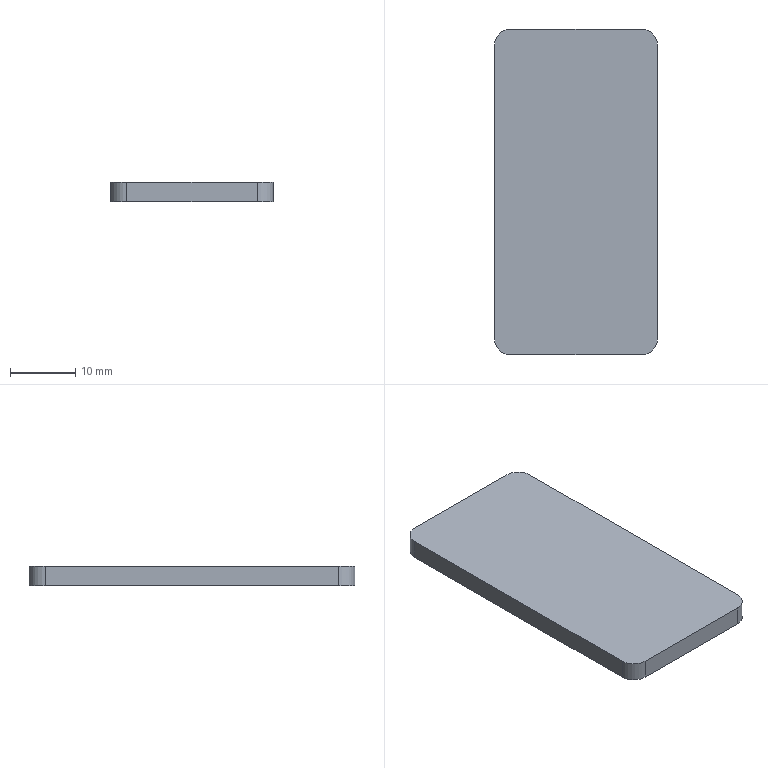Part | STEP file | 7100518 | 1 solid | 10 faces | box 25 x 50 x 3 mm | volume 3734 mm3 | plane 6 | cylinder 4 | commonest cylinder face diameters 5 x4
STEP:
#1=CARTESIAN_POINT('',(0.,0.,0.));
#2=DIRECTION('',(0.,0.,1.));
#3=DIRECTION('',(1.,0.,0.));
#4=AXIS2_PLACEMENT_3D('',#1,#2,#3);
#5=CARTESIAN_POINT('',(10.,-25.,0.));
#6=VERTEX_POINT('',#5);
#7=CARTESIAN_POINT('',(12.5,-22.5,0.));
#8=VERTEX_POINT('',#7);
#9=CARTESIAN_POINT('',(10.,-22.5,0.));
#10=DIRECTION('',(0.,0.,1.));
#11=DIRECTION('',(1.,0.,0.));
#12=AXIS2_PLACEMENT_3D('',#9,#10,#11);
#13=CIRCLE('',#12,2.5);
#14=CARTESIAN_POINT('',(10.,-22.5,3.));
#15=DIRECTION('',(0.,0.,-1.));
#16=DIRECTION('',(-1.,0.,0.));
#17=AXIS2_PLACEMENT_3D('',#14,#15,#16);
#18=CYLINDRICAL_SURFACE('',#17,2.5);
#19=CARTESIAN_POINT('',(9.425,3.));
#20=DIRECTION('',(-1.,0.));
#21=VECTOR('',#20,1.);
#22=LINE('',#19,#21);
#23=(GEOMETRIC_REPRESENTATION_CONTEXT(2)PARAMETRIC_REPRESENTATION_CONTEXT()REPRESENTATION_CONTEXT('',''));
#24=DEFINITIONAL_REPRESENTATION('',(#22),#23);
#25=PCURVE('',#18,#24);
#26=CARTESIAN_POINT('',(10.,-22.5,0.));
#27=DIRECTION('',(0.,0.,1.));
#28=DIRECTION('',(1.,0.,0.));
#29=AXIS2_PLACEMENT_3D('',#26,#27,#28);
#30=PLANE('',#29);
#31=CARTESIAN_POINT('',(0.,0.));
#32=DIRECTION('',(1.,0.));
#33=AXIS2_PLACEMENT_2D('',#31,#32);
#34=CIRCLE('',#33,2.5);
#35=(GEOMETRIC_REPRESENTATION_CONTEXT(2)PARAMETRIC_REPRESENTATION_CONTEXT()REPRESENTATION_CONTEXT('',''));
#36=DEFINITIONAL_REPRESENTATION('',(#34),#35);
#37=PCURVE('',#30,#36);
#38=SURFACE_CURVE('',#13,(#25,#37),.PCURVE_S1.);
#39=EDGE_CURVE('',#6,#8,#38,.T.);
#40=ORIENTED_EDGE('',*,*,#39,.T.);
#41=CARTESIAN_POINT('',(12.5,-22.5,3.));
#42=VERTEX_POINT('',#41);
#43=CARTESIAN_POINT('',(12.5,-22.5,3.));
#44=DIRECTION('',(0.,0.,-1.));
#45=VECTOR('',#44,1.);
#46=LINE('',#43,#45);
#47=CARTESIAN_POINT('',(3.142,0.));
#48=DIRECTION('',(0.,1.));
#49=VECTOR('',#48,1.);
#50=LINE('',#47,#49);
#51=(GEOMETRIC_REPRESENTATION_CONTEXT(2)PARAMETRIC_REPRESENTATION_CONTEXT()REPRESENTATION_CONTEXT('',''));
#52=DEFINITIONAL_REPRESENTATION('',(#50),#51);
#53=PCURVE('',#18,#52);
#54=CARTESIAN_POINT('',(12.5,22.5,3.));
#55=DIRECTION('',(-1.,0.,0.));
#56=DIRECTION('',(0.,-1.,0.));
#57=AXIS2_PLACEMENT_3D('',#54,#55,#56);
#58=PLANE('',#57);
#59=CARTESIAN_POINT('',(45.,0.));
#60=DIRECTION('',(0.,-1.));
#61=VECTOR('',#60,1.);
#62=LINE('',#59,#61);
#63=(GEOMETRIC_REPRESENTATION_CONTEXT(2)PARAMETRIC_REPRESENTATION_CONTEXT()REPRESENTATION_CONTEXT('',''));
#64=DEFINITIONAL_REPRESENTATION('',(#62),#63);
#65=PCURVE('',#58,#64);
#66=SURFACE_CURVE('',#46,(#53,#65),.PCURVE_S1.);
#67=EDGE_CURVE('',#42,#8,#66,.T.);
#68=ORIENTED_EDGE('',*,*,#67,.F.);
#69=CARTESIAN_POINT('',(10.,-25.,3.));
#70=VERTEX_POINT('',#69);
#71=CARTESIAN_POINT('',(10.,-22.5,3.));
#72=DIRECTION('',(0.,0.,1.));
#73=DIRECTION('',(1.,0.,0.));
#74=AXIS2_PLACEMENT_3D('',#71,#72,#73);
#75=CIRCLE('',#74,2.5);
#76=CARTESIAN_POINT('',(9.425,0.));
#77=DIRECTION('',(-1.,0.));
#78=VECTOR('',#77,1.);
#79=LINE('',#76,#78);
#80=(GEOMETRIC_REPRESENTATION_CONTEXT(2)PARAMETRIC_REPRESENTATION_CONTEXT()REPRESENTATION_CONTEXT('',''));
#81=DEFINITIONAL_REPRESENTATION('',(#79),#80);
#82=PCURVE('',#18,#81);
#83=CARTESIAN_POINT('',(10.,-22.5,3.));
#84=DIRECTION('',(0.,0.,1.));
#85=DIRECTION('',(1.,0.,0.));
#86=AXIS2_PLACEMENT_3D('',#83,#84,#85);
#87=PLANE('',#86);
#88=CARTESIAN_POINT('',(0.,0.));
#89=DIRECTION('',(1.,0.));
#90=AXIS2_PLACEMENT_2D('',#88,#89);
#91=CIRCLE('',#90,2.5);
#92=(GEOMETRIC_REPRESENTATION_CONTEXT(2)PARAMETRIC_REPRESENTATION_CONTEXT()REPRESENTATION_CONTEXT('',''));
#93=DEFINITIONAL_REPRESENTATION('',(#91),#92);
#94=PCURVE('',#87,#93);
#95=SURFACE_CURVE('',#75,(#82,#94),.PCURVE_S1.);
#96=EDGE_CURVE('',#70,#42,#95,.T.);
#97=ORIENTED_EDGE('',*,*,#96,.F.);
#98=CARTESIAN_POINT('',(10.,-25.,3.));
#99=DIRECTION('',(0.,0.,-1.));
#100=VECTOR('',#99,1.);
#101=LINE('',#98,#100);
#102=CARTESIAN_POINT('',(4.712,0.));
#103=DIRECTION('',(0.,1.));
#104=VECTOR('',#103,1.);
#105=LINE('',#102,#104);
#106=(GEOMETRIC_REPRESENTATION_CONTEXT(2)PARAMETRIC_REPRESENTATION_CONTEXT()REPRESENTATION_CONTEXT('',''));
#107=DEFINITIONAL_REPRESENTATION('',(#105),#106);
#108=PCURVE('',#18,#107);
#109=CARTESIAN_POINT('',(-10.,-25.,3.));
#110=DIRECTION('',(0.,1.,0.));
#111=DIRECTION('',(-1.,0.,0.));
#112=AXIS2_PLACEMENT_3D('',#109,#110,#111);
#113=PLANE('',#112);
#114=CARTESIAN_POINT('',(-20.,0.));
#115=DIRECTION('',(0.,-1.));
#116=VECTOR('',#115,1.);
#117=LINE('',#114,#116);
#118=(GEOMETRIC_REPRESENTATION_CONTEXT(2)PARAMETRIC_REPRESENTATION_CONTEXT()REPRESENTATION_CONTEXT('',''));
#119=DEFINITIONAL_REPRESENTATION('',(#117),#118);
#120=PCURVE('',#113,#119);
#121=SURFACE_CURVE('',#101,(#108,#120),.PCURVE_S1.);
#122=EDGE_CURVE('',#70,#6,#121,.T.);
#123=ORIENTED_EDGE('',*,*,#122,.T.);
#124=EDGE_LOOP('',(#40,#68,#97,#123));
#125=FACE_BOUND('',#124,.T.);
#126=ADVANCED_FACE('',(#125),#18,.T.);
#127=CARTESIAN_POINT('',(12.5,22.5,0.));
#128=VERTEX_POINT('',#127);
#129=CARTESIAN_POINT('',(12.5,22.5,0.));
#130=DIRECTION('',(0.,1.,0.));
#131=VECTOR('',#130,1.);
#132=LINE('',#129,#131);
#133=CARTESIAN_POINT('',(0.,-3.));
#134=DIRECTION('',(-1.,0.));
#135=VECTOR('',#134,1.);
#136=LINE('',#133,#135);
#137=(GEOMETRIC_REPRESENTATION_CONTEXT(2)PARAMETRIC_REPRESENTATION_CONTEXT()REPRESENTATION_CONTEXT('',''));
#138=DEFINITIONAL_REPRESENTATION('',(#136),#137);
#139=PCURVE('',#58,#138);
#140=CARTESIAN_POINT('',(2.5,45.));
#141=DIRECTION('',(0.,1.));
#142=VECTOR('',#141,1.);
#143=LINE('',#140,#142);
#144=(GEOMETRIC_REPRESENTATION_CONTEXT(2)PARAMETRIC_REPRESENTATION_CONTEXT()REPRESENTATION_CONTEXT('',''));
#145=DEFINITIONAL_REPRESENTATION('',(#143),#144);
#146=PCURVE('',#30,#145);
#147=SURFACE_CURVE('',#132,(#139,#146),.PCURVE_S1.);
#148=EDGE_CURVE('',#8,#128,#147,.T.);
#149=ORIENTED_EDGE('',*,*,#148,.T.);
#150=CARTESIAN_POINT('',(12.5,22.5,3.));
#151=VERTEX_POINT('',#150);
#152=CARTESIAN_POINT('',(12.5,22.5,3.));
#153=DIRECTION('',(0.,0.,-1.));
#154=VECTOR('',#153,1.);
#155=LINE('',#152,#154);
#156=CARTESIAN_POINT('',(0.,0.));
#157=DIRECTION('',(0.,-1.));
#158=VECTOR('',#157,1.);
#159=LINE('',#156,#158);
#160=(GEOMETRIC_REPRESENTATION_CONTEXT(2)PARAMETRIC_REPRESENTATION_CONTEXT()REPRESENTATION_CONTEXT('',''));
#161=DEFINITIONAL_REPRESENTATION('',(#159),#160);
#162=PCURVE('',#58,#161);
#163=CARTESIAN_POINT('',(10.,22.5,3.));
#164=DIRECTION('',(0.,0.,-1.));
#165=DIRECTION('',(-1.,0.,0.));
#166=AXIS2_PLACEMENT_3D('',#163,#164,#165);
#167=CYLINDRICAL_SURFACE('',#166,2.5);
#168=CARTESIAN_POINT('',(3.142,0.));
#169=DIRECTION('',(0.,1.));
#170=VECTOR('',#169,1.);
#171=LINE('',#168,#170);
#172=(GEOMETRIC_REPRESENTATION_CONTEXT(2)PARAMETRIC_REPRESENTATION_CONTEXT()REPRESENTATION_CONTEXT('',''));
#173=DEFINITIONAL_REPRESENTATION('',(#171),#172);
#174=PCURVE('',#167,#173);
#175=SURFACE_CURVE('',#155,(#162,#174),.PCURVE_S1.);
#176=EDGE_CURVE('',#151,#128,#175,.T.);
#177=ORIENTED_EDGE('',*,*,#176,.F.);
#178=CARTESIAN_POINT('',(12.5,22.5,3.));
#179=DIRECTION('',(0.,1.,0.));
#180=VECTOR('',#179,1.);
#181=LINE('',#178,#180);
#182=CARTESIAN_POINT('',(0.,0.));
#183=DIRECTION('',(-1.,0.));
#184=VECTOR('',#183,1.);
#185=LINE('',#182,#184);
#186=(GEOMETRIC_REPRESENTATION_CONTEXT(2)PARAMETRIC_REPRESENTATION_CONTEXT()REPRESENTATION_CONTEXT('',''));
#187=DEFINITIONAL_REPRESENTATION('',(#185),#186);
#188=PCURVE('',#58,#187);
#189=CARTESIAN_POINT('',(2.5,45.));
#190=DIRECTION('',(0.,1.));
#191=VECTOR('',#190,1.);
#192=LINE('',#189,#191);
#193=(GEOMETRIC_REPRESENTATION_CONTEXT(2)PARAMETRIC_REPRESENTATION_CONTEXT()REPRESENTATION_CONTEXT('',''));
#194=DEFINITIONAL_REPRESENTATION('',(#192),#193);
#195=PCURVE('',#87,#194);
#196=SURFACE_CURVE('',#181,(#188,#195),.PCURVE_S1.);
#197=EDGE_CURVE('',#42,#151,#196,.T.);
#198=ORIENTED_EDGE('',*,*,#197,.F.);
#199=ORIENTED_EDGE('',*,*,#67,.T.);
#200=EDGE_LOOP('',(#149,#177,#198,#199));
#201=FACE_BOUND('',#200,.T.);
#202=ADVANCED_FACE('',(#201),#58,.F.);
#203=CARTESIAN_POINT('',(10.,25.,0.));
#204=VERTEX_POINT('',#203);
#205=CARTESIAN_POINT('',(10.,22.5,0.));
#206=DIRECTION('',(0.,0.,1.));
#207=DIRECTION('',(-1.,0.,0.));
#208=AXIS2_PLACEMENT_3D('',#205,#206,#207);
#209=CIRCLE('',#208,2.5);
#210=CARTESIAN_POINT('',(6.283,3.));
#211=DIRECTION('',(-1.,0.));
#212=VECTOR('',#211,1.);
#213=LINE('',#210,#212);
#214=(GEOMETRIC_REPRESENTATION_CONTEXT(2)PARAMETRIC_REPRESENTATION_CONTEXT()REPRESENTATION_CONTEXT('',''));
#215=DEFINITIONAL_REPRESENTATION('',(#213),#214);
#216=PCURVE('',#167,#215);
#217=CARTESIAN_POINT('',(0.,45.));
#218=DIRECTION('',(-1.,0.));
#219=AXIS2_PLACEMENT_2D('',#217,#218);
#220=CIRCLE('',#219,2.5);
#221=(GEOMETRIC_REPRESENTATION_CONTEXT(2)PARAMETRIC_REPRESENTATION_CONTEXT()REPRESENTATION_CONTEXT('',''));
#222=DEFINITIONAL_REPRESENTATION('',(#220),#221);
#223=PCURVE('',#30,#222);
#224=SURFACE_CURVE('',#209,(#216,#223),.PCURVE_S1.);
#225=EDGE_CURVE('',#128,#204,#224,.T.);
#226=ORIENTED_EDGE('',*,*,#225,.T.);
#227=CARTESIAN_POINT('',(10.,25.,3.));
#228=VERTEX_POINT('',#227);
#229=CARTESIAN_POINT('',(10.,25.,3.));
#230=DIRECTION('',(0.,0.,-1.));
#231=VECTOR('',#230,1.);
#232=LINE('',#229,#231);
#233=CARTESIAN_POINT('',(1.571,0.));
#234=DIRECTION('',(0.,1.));
#235=VECTOR('',#234,1.);
#236=LINE('',#233,#235);
#237=(GEOMETRIC_REPRESENTATION_CONTEXT(2)PARAMETRIC_REPRESENTATION_CONTEXT()REPRESENTATION_CONTEXT('',''));
#238=DEFINITIONAL_REPRESENTATION('',(#236),#237);
#239=PCURVE('',#167,#238);
#240=CARTESIAN_POINT('',(-10.,25.,3.));
#241=DIRECTION('',(0.,-1.,0.));
#242=DIRECTION('',(0.,0.,-1.));
#243=AXIS2_PLACEMENT_3D('',#240,#241,#242);
#244=PLANE('',#243);
#245=CARTESIAN_POINT('',(0.,20.));
#246=DIRECTION('',(1.,0.));
#247=VECTOR('',#246,1.);
#248=LINE('',#245,#247);
#249=(GEOMETRIC_REPRESENTATION_CONTEXT(2)PARAMETRIC_REPRESENTATION_CONTEXT()REPRESENTATION_CONTEXT('',''));
#250=DEFINITIONAL_REPRESENTATION('',(#248),#249);
#251=PCURVE('',#244,#250);
#252=SURFACE_CURVE('',#232,(#239,#251),.PCURVE_S1.);
#253=EDGE_CURVE('',#228,#204,#252,.T.);
#254=ORIENTED_EDGE('',*,*,#253,.F.);
#255=CARTESIAN_POINT('',(10.,22.5,3.));
#256=DIRECTION('',(0.,0.,1.));
#257=DIRECTION('',(-1.,0.,0.));
#258=AXIS2_PLACEMENT_3D('',#255,#256,#257);
#259=CIRCLE('',#258,2.5);
#260=CARTESIAN_POINT('',(6.283,0.));
#261=DIRECTION('',(-1.,0.));
#262=VECTOR('',#261,1.);
#263=LINE('',#260,#262);
#264=(GEOMETRIC_REPRESENTATION_CONTEXT(2)PARAMETRIC_REPRESENTATION_CONTEXT()REPRESENTATION_CONTEXT('',''));
#265=DEFINITIONAL_REPRESENTATION('',(#263),#264);
#266=PCURVE('',#167,#265);
#267=CARTESIAN_POINT('',(0.,45.));
#268=DIRECTION('',(-1.,0.));
#269=AXIS2_PLACEMENT_2D('',#267,#268);
#270=CIRCLE('',#269,2.5);
#271=(GEOMETRIC_REPRESENTATION_CONTEXT(2)PARAMETRIC_REPRESENTATION_CONTEXT()REPRESENTATION_CONTEXT('',''));
#272=DEFINITIONAL_REPRESENTATION('',(#270),#271);
#273=PCURVE('',#87,#272);
#274=SURFACE_CURVE('',#259,(#266,#273),.PCURVE_S1.);
#275=EDGE_CURVE('',#151,#228,#274,.T.);
#276=ORIENTED_EDGE('',*,*,#275,.F.);
#277=ORIENTED_EDGE('',*,*,#176,.T.);
#278=EDGE_LOOP('',(#226,#254,#276,#277));
#279=FACE_BOUND('',#278,.T.);
#280=ADVANCED_FACE('',(#279),#167,.T.);
#281=CARTESIAN_POINT('',(-10.,25.,0.));
#282=VERTEX_POINT('',#281);
#283=CARTESIAN_POINT('',(-10.,25.,0.));
#284=DIRECTION('',(-1.,0.,0.));
#285=VECTOR('',#284,1.);
#286=LINE('',#283,#285);
#287=CARTESIAN_POINT('',(3.,0.));
#288=DIRECTION('',(0.,-1.));
#289=VECTOR('',#288,1.);
#290=LINE('',#287,#289);
#291=(GEOMETRIC_REPRESENTATION_CONTEXT(2)PARAMETRIC_REPRESENTATION_CONTEXT()REPRESENTATION_CONTEXT('',''));
#292=DEFINITIONAL_REPRESENTATION('',(#290),#291);
#293=PCURVE('',#244,#292);
#294=CARTESIAN_POINT('',(-20.,47.5));
#295=DIRECTION('',(-1.,0.));
#296=VECTOR('',#295,1.);
#297=LINE('',#294,#296);
#298=(GEOMETRIC_REPRESENTATION_CONTEXT(2)PARAMETRIC_REPRESENTATION_CONTEXT()REPRESENTATION_CONTEXT('',''));
#299=DEFINITIONAL_REPRESENTATION('',(#297),#298);
#300=PCURVE('',#30,#299);
#301=SURFACE_CURVE('',#286,(#293,#300),.PCURVE_S1.);
#302=EDGE_CURVE('',#204,#282,#301,.T.);
#303=ORIENTED_EDGE('',*,*,#302,.T.);
#304=CARTESIAN_POINT('',(-10.,25.,3.));
#305=VERTEX_POINT('',#304);
#306=CARTESIAN_POINT('',(-10.,25.,3.));
#307=DIRECTION('',(0.,0.,-1.));
#308=VECTOR('',#307,1.);
#309=LINE('',#306,#308);
#310=CARTESIAN_POINT('',(0.,0.));
#311=DIRECTION('',(1.,0.));
#312=VECTOR('',#311,1.);
#313=LINE('',#310,#312);
#314=(GEOMETRIC_REPRESENTATION_CONTEXT(2)PARAMETRIC_REPRESENTATION_CONTEXT()REPRESENTATION_CONTEXT('',''));
#315=DEFINITIONAL_REPRESENTATION('',(#313),#314);
#316=PCURVE('',#244,#315);
#317=CARTESIAN_POINT('',(-10.,22.5,3.));
#318=DIRECTION('',(0.,0.,-1.));
#319=DIRECTION('',(-1.,0.,0.));
#320=AXIS2_PLACEMENT_3D('',#317,#318,#319);
#321=CYLINDRICAL_SURFACE('',#320,2.5);
#322=CARTESIAN_POINT('',(1.571,0.));
#323=DIRECTION('',(0.,1.));
#324=VECTOR('',#323,1.);
#325=LINE('',#322,#324);
#326=(GEOMETRIC_REPRESENTATION_CONTEXT(2)PARAMETRIC_REPRESENTATION_CONTEXT()REPRESENTATION_CONTEXT('',''));
#327=DEFINITIONAL_REPRESENTATION('',(#325),#326);
#328=PCURVE('',#321,#327);
#329=SURFACE_CURVE('',#309,(#316,#328),.PCURVE_S1.);
#330=EDGE_CURVE('',#305,#282,#329,.T.);
#331=ORIENTED_EDGE('',*,*,#330,.F.);
#332=CARTESIAN_POINT('',(-10.,25.,3.));
#333=DIRECTION('',(-1.,0.,0.));
#334=VECTOR('',#333,1.);
#335=LINE('',#332,#334);
#336=CARTESIAN_POINT('',(0.,0.));
#337=DIRECTION('',(0.,-1.));
#338=VECTOR('',#337,1.);
#339=LINE('',#336,#338);
#340=(GEOMETRIC_REPRESENTATION_CONTEXT(2)PARAMETRIC_REPRESENTATION_CONTEXT()REPRESENTATION_CONTEXT('',''));
#341=DEFINITIONAL_REPRESENTATION('',(#339),#340);
#342=PCURVE('',#244,#341);
#343=CARTESIAN_POINT('',(-20.,47.5));
#344=DIRECTION('',(-1.,0.));
#345=VECTOR('',#344,1.);
#346=LINE('',#343,#345);
#347=(GEOMETRIC_REPRESENTATION_CONTEXT(2)PARAMETRIC_REPRESENTATION_CONTEXT()REPRESENTATION_CONTEXT('',''));
#348=DEFINITIONAL_REPRESENTATION('',(#346),#347);
#349=PCURVE('',#87,#348);
#350=SURFACE_CURVE('',#335,(#342,#349),.PCURVE_S1.);
#351=EDGE_CURVE('',#228,#305,#350,.T.);
#352=ORIENTED_EDGE('',*,*,#351,.F.);
#353=ORIENTED_EDGE('',*,*,#253,.T.);
#354=EDGE_LOOP('',(#303,#331,#352,#353));
#355=FACE_BOUND('',#354,.T.);
#356=ADVANCED_FACE('',(#355),#244,.F.);
#357=CARTESIAN_POINT('',(-12.5,22.5,0.));
#358=VERTEX_POINT('',#357);
#359=CARTESIAN_POINT('',(-10.,22.5,0.));
#360=DIRECTION('',(0.,0.,1.));
#361=DIRECTION('',(1.,0.,0.));
#362=AXIS2_PLACEMENT_3D('',#359,#360,#361);
#363=CIRCLE('',#362,2.5);
#364=CARTESIAN_POINT('',(3.142,3.));
#365=DIRECTION('',(-1.,0.));
#366=VECTOR('',#365,1.);
#367=LINE('',#364,#366);
#368=(GEOMETRIC_REPRESENTATION_CONTEXT(2)PARAMETRIC_REPRESENTATION_CONTEXT()REPRESENTATION_CONTEXT('',''));
#369=DEFINITIONAL_REPRESENTATION('',(#367),#368);
#370=PCURVE('',#321,#369);
#371=CARTESIAN_POINT('',(-20.,45.));
#372=DIRECTION('',(1.,0.));
#373=AXIS2_PLACEMENT_2D('',#371,#372);
#374=CIRCLE('',#373,2.5);
#375=(GEOMETRIC_REPRESENTATION_CONTEXT(2)PARAMETRIC_REPRESENTATION_CONTEXT()REPRESENTATION_CONTEXT('',''));
#376=DEFINITIONAL_REPRESENTATION('',(#374),#375);
#377=PCURVE('',#30,#376);
#378=SURFACE_CURVE('',#363,(#370,#377),.PCURVE_S1.);
#379=EDGE_CURVE('',#282,#358,#378,.T.);
#380=ORIENTED_EDGE('',*,*,#379,.T.);
#381=CARTESIAN_POINT('',(-12.5,22.5,3.));
#382=VERTEX_POINT('',#381);
#383=CARTESIAN_POINT('',(-12.5,22.5,3.));
#384=DIRECTION('',(0.,0.,-1.));
#385=VECTOR('',#384,1.);
#386=LINE('',#383,#385);
#387=CARTESIAN_POINT('',(0.,0.));
#388=DIRECTION('',(0.,1.));
#389=VECTOR('',#388,1.);
#390=LINE('',#387,#389);
#391=(GEOMETRIC_REPRESENTATION_CONTEXT(2)PARAMETRIC_REPRESENTATION_CONTEXT()REPRESENTATION_CONTEXT('',''));
#392=DEFINITIONAL_REPRESENTATION('',(#390),#391);
#393=PCURVE('',#321,#392);
#394=CARTESIAN_POINT('',(-12.5,22.5,3.));
#395=DIRECTION('',(1.,0.,0.));
#396=DIRECTION('',(0.,1.,0.));
#397=AXIS2_PLACEMENT_3D('',#394,#395,#396);
#398=PLANE('',#397);
#399=CARTESIAN_POINT('',(0.,0.));
#400=DIRECTION('',(0.,-1.));
#401=VECTOR('',#400,1.);
#402=LINE('',#399,#401);
#403=(GEOMETRIC_REPRESENTATION_CONTEXT(2)PARAMETRIC_REPRESENTATION_CONTEXT()REPRESENTATION_CONTEXT('',''));
#404=DEFINITIONAL_REPRESENTATION('',(#402),#403);
#405=PCURVE('',#398,#404);
#406=SURFACE_CURVE('',#386,(#393,#405),.PCURVE_S1.);
#407=EDGE_CURVE('',#382,#358,#406,.T.);
#408=ORIENTED_EDGE('',*,*,#407,.F.);
#409=CARTESIAN_POINT('',(-10.,22.5,3.));
#410=DIRECTION('',(0.,0.,1.));
#411=DIRECTION('',(1.,0.,0.));
#412=AXIS2_PLACEMENT_3D('',#409,#410,#411);
#413=CIRCLE('',#412,2.5);
#414=CARTESIAN_POINT('',(3.142,0.));
#415=DIRECTION('',(-1.,0.));
#416=VECTOR('',#415,1.);
#417=LINE('',#414,#416);
#418=(GEOMETRIC_REPRESENTATION_CONTEXT(2)PARAMETRIC_REPRESENTATION_CONTEXT()REPRESENTATION_CONTEXT('',''));
#419=DEFINITIONAL_REPRESENTATION('',(#417),#418);
#420=PCURVE('',#321,#419);
#421=CARTESIAN_POINT('',(-20.,45.));
#422=DIRECTION('',(1.,0.));
#423=AXIS2_PLACEMENT_2D('',#421,#422);
#424=CIRCLE('',#423,2.5);
#425=(GEOMETRIC_REPRESENTATION_CONTEXT(2)PARAMETRIC_REPRESENTATION_CONTEXT()REPRESENTATION_CONTEXT('',''));
#426=DEFINITIONAL_REPRESENTATION('',(#424),#425);
#427=PCURVE('',#87,#426);
#428=SURFACE_CURVE('',#413,(#420,#427),.PCURVE_S1.);
#429=EDGE_CURVE('',#305,#382,#428,.T.);
#430=ORIENTED_EDGE('',*,*,#429,.F.);
#431=ORIENTED_EDGE('',*,*,#330,.T.);
#432=EDGE_LOOP('',(#380,#408,#430,#431));
#433=FACE_BOUND('',#432,.T.);
#434=ADVANCED_FACE('',(#433),#321,.T.);
#435=CARTESIAN_POINT('',(-12.5,-22.5,0.));
#436=VERTEX_POINT('',#435);
#437=CARTESIAN_POINT('',(-12.5,22.5,0.));
#438=DIRECTION('',(0.,-1.,0.));
#439=VECTOR('',#438,1.);
#440=LINE('',#437,#439);
#441=CARTESIAN_POINT('',(0.,-3.));
#442=DIRECTION('',(-1.,0.));
#443=VECTOR('',#442,1.);
#444=LINE('',#441,#443);
#445=(GEOMETRIC_REPRESENTATION_CONTEXT(2)PARAMETRIC_REPRESENTATION_CONTEXT()REPRESENTATION_CONTEXT('',''));
#446=DEFINITIONAL_REPRESENTATION('',(#444),#445);
#447=PCURVE('',#398,#446);
#448=CARTESIAN_POINT('',(-22.5,45.));
#449=DIRECTION('',(0.,-1.));
#450=VECTOR('',#449,1.);
#451=LINE('',#448,#450);
#452=(GEOMETRIC_REPRESENTATION_CONTEXT(2)PARAMETRIC_REPRESENTATION_CONTEXT()REPRESENTATION_CONTEXT('',''));
#453=DEFINITIONAL_REPRESENTATION('',(#451),#452);
#454=PCURVE('',#30,#453);
#455=SURFACE_CURVE('',#440,(#447,#454),.PCURVE_S1.);
#456=EDGE_CURVE('',#358,#436,#455,.T.);
#457=ORIENTED_EDGE('',*,*,#456,.T.);
#458=CARTESIAN_POINT('',(-12.5,-22.5,3.));
#459=VERTEX_POINT('',#458);
#460=CARTESIAN_POINT('',(-12.5,-22.5,3.));
#461=DIRECTION('',(0.,0.,-1.));
#462=VECTOR('',#461,1.);
#463=LINE('',#460,#462);
#464=CARTESIAN_POINT('',(-45.,0.));
#465=DIRECTION('',(0.,-1.));
#466=VECTOR('',#465,1.);
#467=LINE('',#464,#466);
#468=(GEOMETRIC_REPRESENTATION_CONTEXT(2)PARAMETRIC_REPRESENTATION_CONTEXT()REPRESENTATION_CONTEXT('',''));
#469=DEFINITIONAL_REPRESENTATION('',(#467),#468);
#470=PCURVE('',#398,#469);
#471=CARTESIAN_POINT('',(-10.,-22.5,3.));
#472=DIRECTION('',(0.,0.,-1.));
#473=DIRECTION('',(-1.,0.,0.));
#474=AXIS2_PLACEMENT_3D('',#471,#472,#473);
#475=CYLINDRICAL_SURFACE('',#474,2.5);
#476=CARTESIAN_POINT('',(6.283,0.));
#477=DIRECTION('',(0.,1.));
#478=VECTOR('',#477,1.);
#479=LINE('',#476,#478);
#480=(GEOMETRIC_REPRESENTATION_CONTEXT(2)PARAMETRIC_REPRESENTATION_CONTEXT()REPRESENTATION_CONTEXT('',''));
#481=DEFINITIONAL_REPRESENTATION('',(#479),#480);
#482=PCURVE('',#475,#481);
#483=SURFACE_CURVE('',#463,(#470,#482),.PCURVE_S1.);
#484=EDGE_CURVE('',#459,#436,#483,.T.);
#485=ORIENTED_EDGE('',*,*,#484,.F.);
#486=CARTESIAN_POINT('',(-12.5,22.5,3.));
#487=DIRECTION('',(0.,-1.,0.));
#488=VECTOR('',#487,1.);
#489=LINE('',#486,#488);
#490=CARTESIAN_POINT('',(0.,0.));
#491=DIRECTION('',(-1.,0.));
#492=VECTOR('',#491,1.);
#493=LINE('',#490,#492);
#494=(GEOMETRIC_REPRESENTATION_CONTEXT(2)PARAMETRIC_REPRESENTATION_CONTEXT()REPRESENTATION_CONTEXT('',''));
#495=DEFINITIONAL_REPRESENTATION('',(#493),#494);
#496=PCURVE('',#398,#495);
#497=CARTESIAN_POINT('',(-22.5,45.));
#498=DIRECTION('',(0.,-1.));
#499=VECTOR('',#498,1.);
#500=LINE('',#497,#499);
#501=(GEOMETRIC_REPRESENTATION_CONTEXT(2)PARAMETRIC_REPRESENTATION_CONTEXT()REPRESENTATION_CONTEXT('',''));
#502=DEFINITIONAL_REPRESENTATION('',(#500),#501);
#503=PCURVE('',#87,#502);
#504=SURFACE_CURVE('',#489,(#496,#503),.PCURVE_S1.);
#505=EDGE_CURVE('',#382,#459,#504,.T.);
#506=ORIENTED_EDGE('',*,*,#505,.F.);
#507=ORIENTED_EDGE('',*,*,#407,.T.);
#508=EDGE_LOOP('',(#457,#485,#506,#507));
#509=FACE_BOUND('',#508,.T.);
#510=ADVANCED_FACE('',(#509),#398,.F.);
#511=CARTESIAN_POINT('',(-10.,-25.,0.));
#512=VERTEX_POINT('',#511);
#513=CARTESIAN_POINT('',(-10.,-22.5,0.));
#514=DIRECTION('',(0.,0.,1.));
#515=DIRECTION('',(1.,0.,0.));
#516=AXIS2_PLACEMENT_3D('',#513,#514,#515);
#517=CIRCLE('',#516,2.5);
#518=CARTESIAN_POINT('',(9.425,3.));
#519=DIRECTION('',(-1.,0.));
#520=VECTOR('',#519,1.);
#521=LINE('',#518,#520);
#522=(GEOMETRIC_REPRESENTATION_CONTEXT(2)PARAMETRIC_REPRESENTATION_CONTEXT()REPRESENTATION_CONTEXT('',''));
#523=DEFINITIONAL_REPRESENTATION('',(#521),#522);
#524=PCURVE('',#475,#523);
#525=CARTESIAN_POINT('',(-20.,0.));
#526=DIRECTION('',(1.,0.));
#527=AXIS2_PLACEMENT_2D('',#525,#526);
#528=CIRCLE('',#527,2.5);
#529=(GEOMETRIC_REPRESENTATION_CONTEXT(2)PARAMETRIC_REPRESENTATION_CONTEXT()REPRESENTATION_CONTEXT('',''));
#530=DEFINITIONAL_REPRESENTATION('',(#528),#529);
#531=PCURVE('',#30,#530);
#532=SURFACE_CURVE('',#517,(#524,#531),.PCURVE_S1.);
#533=EDGE_CURVE('',#436,#512,#532,.T.);
#534=ORIENTED_EDGE('',*,*,#533,.T.);
#535=CARTESIAN_POINT('',(-10.,-25.,3.));
#536=VERTEX_POINT('',#535);
#537=CARTESIAN_POINT('',(-10.,-25.,3.));
#538=DIRECTION('',(0.,0.,-1.));
#539=VECTOR('',#538,1.);
#540=LINE('',#537,#539);
#541=CARTESIAN_POINT('',(4.712,0.));
#542=DIRECTION('',(0.,1.));
#543=VECTOR('',#542,1.);
#544=LINE('',#541,#543);
#545=(GEOMETRIC_REPRESENTATION_CONTEXT(2)PARAMETRIC_REPRESENTATION_CONTEXT()REPRESENTATION_CONTEXT('',''));
#546=DEFINITIONAL_REPRESENTATION('',(#544),#545);
#547=PCURVE('',#475,#546);
#548=CARTESIAN_POINT('',(0.,0.));
#549=DIRECTION('',(0.,-1.));
#550=VECTOR('',#549,1.);
#551=LINE('',#548,#550);
#552=(GEOMETRIC_REPRESENTATION_CONTEXT(2)PARAMETRIC_REPRESENTATION_CONTEXT()REPRESENTATION_CONTEXT('',''));
#553=DEFINITIONAL_REPRESENTATION('',(#551),#552);
#554=PCURVE('',#113,#553);
#555=SURFACE_CURVE('',#540,(#547,#554),.PCURVE_S1.);
#556=EDGE_CURVE('',#536,#512,#555,.T.);
#557=ORIENTED_EDGE('',*,*,#556,.F.);
#558=CARTESIAN_POINT('',(-10.,-22.5,3.));
#559=DIRECTION('',(0.,0.,1.));
#560=DIRECTION('',(1.,0.,0.));
#561=AXIS2_PLACEMENT_3D('',#558,#559,#560);
#562=CIRCLE('',#561,2.5);
#563=CARTESIAN_POINT('',(9.425,0.));
#564=DIRECTION('',(-1.,0.));
#565=VECTOR('',#564,1.);
#566=LINE('',#563,#565);
#567=(GEOMETRIC_REPRESENTATION_CONTEXT(2)PARAMETRIC_REPRESENTATION_CONTEXT()REPRESENTATION_CONTEXT('',''));
#568=DEFINITIONAL_REPRESENTATION('',(#566),#567);
#569=PCURVE('',#475,#568);
#570=CARTESIAN_POINT('',(-20.,0.));
#571=DIRECTION('',(1.,0.));
#572=AXIS2_PLACEMENT_2D('',#570,#571);
#573=CIRCLE('',#572,2.5);
#574=(GEOMETRIC_REPRESENTATION_CONTEXT(2)PARAMETRIC_REPRESENTATION_CONTEXT()REPRESENTATION_CONTEXT('',''));
#575=DEFINITIONAL_REPRESENTATION('',(#573),#574);
#576=PCURVE('',#87,#575);
#577=SURFACE_CURVE('',#562,(#569,#576),.PCURVE_S1.);
#578=EDGE_CURVE('',#459,#536,#577,.T.);
#579=ORIENTED_EDGE('',*,*,#578,.F.);
#580=ORIENTED_EDGE('',*,*,#484,.T.);
#581=EDGE_LOOP('',(#534,#557,#579,#580));
#582=FACE_BOUND('',#581,.T.);
#583=ADVANCED_FACE('',(#582),#475,.T.);
#584=CARTESIAN_POINT('',(-10.,-25.,0.));
#585=DIRECTION('',(1.,0.,0.));
#586=VECTOR('',#585,1.);
#587=LINE('',#584,#586);
#588=CARTESIAN_POINT('',(0.,-3.));
#589=DIRECTION('',(-1.,0.));
#590=VECTOR('',#589,1.);
#591=LINE('',#588,#590);
#592=(GEOMETRIC_REPRESENTATION_CONTEXT(2)PARAMETRIC_REPRESENTATION_CONTEXT()REPRESENTATION_CONTEXT('',''));
#593=DEFINITIONAL_REPRESENTATION('',(#591),#592);
#594=PCURVE('',#113,#593);
#595=CARTESIAN_POINT('',(-20.,-2.5));
#596=DIRECTION('',(1.,0.));
#597=VECTOR('',#596,1.);
#598=LINE('',#595,#597);
#599=(GEOMETRIC_REPRESENTATION_CONTEXT(2)PARAMETRIC_REPRESENTATION_CONTEXT()REPRESENTATION_CONTEXT('',''));
#600=DEFINITIONAL_REPRESENTATION('',(#598),#599);
#601=PCURVE('',#30,#600);
#602=SURFACE_CURVE('',#587,(#594,#601),.PCURVE_S1.);
#603=EDGE_CURVE('',#512,#6,#602,.T.);
#604=ORIENTED_EDGE('',*,*,#603,.T.);
#605=ORIENTED_EDGE('',*,*,#122,.F.);
#606=CARTESIAN_POINT('',(-10.,-25.,3.));
#607=DIRECTION('',(1.,0.,0.));
#608=VECTOR('',#607,1.);
#609=LINE('',#606,#608);
#610=CARTESIAN_POINT('',(0.,0.));
#611=DIRECTION('',(-1.,0.));
#612=VECTOR('',#611,1.);
#613=LINE('',#610,#612);
#614=(GEOMETRIC_REPRESENTATION_CONTEXT(2)PARAMETRIC_REPRESENTATION_CONTEXT()REPRESENTATION_CONTEXT('',''));
#615=DEFINITIONAL_REPRESENTATION('',(#613),#614);
#616=PCURVE('',#113,#615);
#617=CARTESIAN_POINT('',(-20.,-2.5));
#618=DIRECTION('',(1.,0.));
#619=VECTOR('',#618,1.);
#620=LINE('',#617,#619);
#621=(GEOMETRIC_REPRESENTATION_CONTEXT(2)PARAMETRIC_REPRESENTATION_CONTEXT()REPRESENTATION_CONTEXT('',''));
#622=DEFINITIONAL_REPRESENTATION('',(#620),#621);
#623=PCURVE('',#87,#622);
#624=SURFACE_CURVE('',#609,(#616,#623),.PCURVE_S1.);
#625=EDGE_CURVE('',#536,#70,#624,.T.);
#626=ORIENTED_EDGE('',*,*,#625,.F.);
#627=ORIENTED_EDGE('',*,*,#556,.T.);
#628=EDGE_LOOP('',(#604,#605,#626,#627));
#629=FACE_BOUND('',#628,.T.);
#630=ADVANCED_FACE('',(#629),#113,.F.);
#631=ORIENTED_EDGE('',*,*,#96,.T.);
#632=ORIENTED_EDGE('',*,*,#197,.T.);
#633=ORIENTED_EDGE('',*,*,#275,.T.);
#634=ORIENTED_EDGE('',*,*,#351,.T.);
#635=ORIENTED_EDGE('',*,*,#429,.T.);
#636=ORIENTED_EDGE('',*,*,#505,.T.);
#637=ORIENTED_EDGE('',*,*,#578,.T.);
#638=ORIENTED_EDGE('',*,*,#625,.T.);
#639=EDGE_LOOP('',(#631,#632,#633,#634,#635,#636,#637,#638));
#640=FACE_BOUND('',#639,.T.);
#641=ADVANCED_FACE('',(#640),#87,.T.);
#642=ORIENTED_EDGE('',*,*,#39,.F.);
#643=ORIENTED_EDGE('',*,*,#603,.F.);
#644=ORIENTED_EDGE('',*,*,#533,.F.);
#645=ORIENTED_EDGE('',*,*,#456,.F.);
#646=ORIENTED_EDGE('',*,*,#379,.F.);
#647=ORIENTED_EDGE('',*,*,#302,.F.);
#648=ORIENTED_EDGE('',*,*,#225,.F.);
#649=ORIENTED_EDGE('',*,*,#148,.F.);
#650=EDGE_LOOP('',(#642,#643,#644,#645,#646,#647,#648,#649));
#651=FACE_BOUND('',#650,.T.);
#652=ADVANCED_FACE('',(#651),#30,.F.);
#653=CLOSED_SHELL('',(#126,#202,#280,#356,#434,#510,#583,#630,#641,#652));
#654=MANIFOLD_SOLID_BREP('',#653);
#655=(LENGTH_UNIT()NAMED_UNIT(*)SI_UNIT(.MILLI.,.METRE.));
#656=UNCERTAINTY_MEASURE_WITH_UNIT(LENGTH_MEASURE(0.0000001),#655,'','');
#657=(NAMED_UNIT(*)PLANE_ANGLE_UNIT()SI_UNIT($,.RADIAN.));
#658=(NAMED_UNIT(*)SI_UNIT($,.STERADIAN.)SOLID_ANGLE_UNIT());
#659=(GEOMETRIC_REPRESENTATION_CONTEXT(3)GLOBAL_UNCERTAINTY_ASSIGNED_CONTEXT((#656))GLOBAL_UNIT_ASSIGNED_CONTEXT((#655,#657,#658))REPRESENTATION_CONTEXT('',''));
#660=ADVANCED_BREP_SHAPE_REPRESENTATION('',(#4,#654),#659);